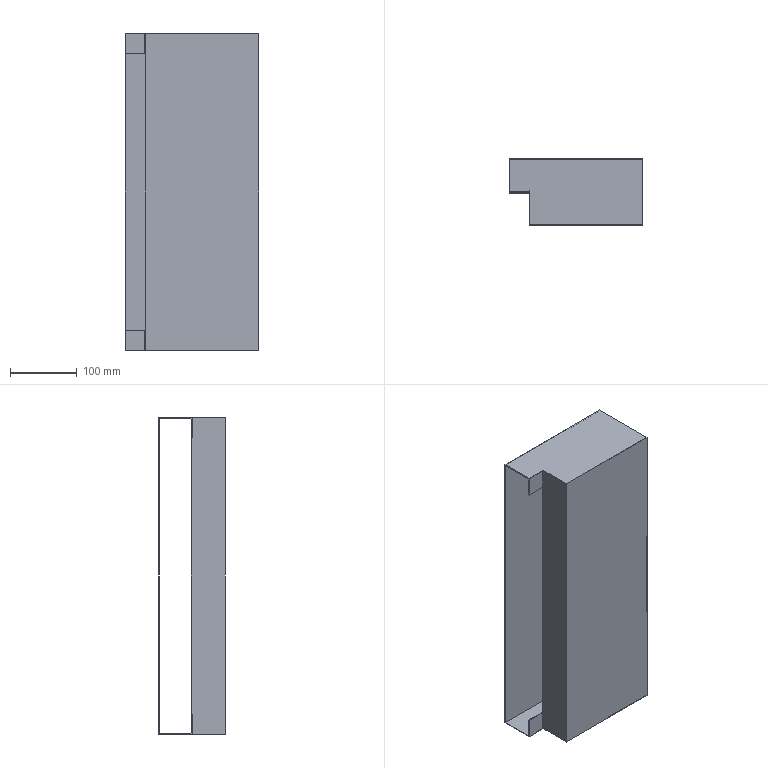Part | SolidWorks | features BaseBody 1 | 1 solid | 23 faces | box 200 x 100 x 472.4 mm | volume 283368 mm3 | plane 23
STEP:
#1=CARTESIAN_POINT('',(-200.,48.8,-236.2));
#2=VERTEX_POINT('',#1);
#3=CARTESIAN_POINT('',(-171.,48.8,-236.2));
#4=VERTEX_POINT('',#3);
#5=CARTESIAN_POINT('',(-171.,48.8,-236.2));
#6=DIRECTION('',(1.,0.,0.));
#7=VECTOR('',#6,1000.);
#8=LINE('',#5,#7);
#9=EDGE_CURVE('',#2,#4,#8,.T.);
#10=ORIENTED_EDGE('',*,*,#9,.T.);
#11=CARTESIAN_POINT('',(-171.,48.8,-206.2));
#12=VERTEX_POINT('',#11);
#13=CARTESIAN_POINT('',(-171.,48.8,-236.2));
#14=DIRECTION('',(0.,0.,1.));
#15=VECTOR('',#14,1000.);
#16=LINE('',#13,#15);
#17=EDGE_CURVE('',#4,#12,#16,.T.);
#18=ORIENTED_EDGE('',*,*,#17,.T.);
#19=CARTESIAN_POINT('',(-200.,48.8,-206.2));
#20=VERTEX_POINT('',#19);
#21=CARTESIAN_POINT('',(-171.,48.8,-206.2));
#22=DIRECTION('',(-1.,0.,0.));
#23=VECTOR('',#22,1000.);
#24=LINE('',#21,#23);
#25=EDGE_CURVE('',#12,#20,#24,.T.);
#26=ORIENTED_EDGE('',*,*,#25,.T.);
#27=CARTESIAN_POINT('',(-200.,48.8,-236.2));
#28=DIRECTION('',(0.,0.,-1.));
#29=VECTOR('',#28,1000.);
#30=LINE('',#27,#29);
#31=EDGE_CURVE('',#20,#2,#30,.T.);
#32=ORIENTED_EDGE('',*,*,#31,.T.);
#33=EDGE_LOOP('',(#10,#18,#26,#32));
#34=FACE_OUTER_BOUND('',#33,.T.);
#35=CARTESIAN_POINT('',(0.,48.8,0.));
#36=DIRECTION('',(0.,1.,0.));
#37=DIRECTION('',(1.,0.,0.));
#38=AXIS2_PLACEMENT_3D('',#35,#36,#37);
#39=PLANE('',#38);
#40=ADVANCED_FACE('',(#34),#39,.F.);
#41=CARTESIAN_POINT('',(-171.,50.,-206.2));
#42=VERTEX_POINT('',#41);
#43=CARTESIAN_POINT('',(-200.,50.,-206.2));
#44=VERTEX_POINT('',#43);
#45=CARTESIAN_POINT('',(-171.,50.,-206.2));
#46=DIRECTION('',(-1.,0.,0.));
#47=VECTOR('',#46,1000.);
#48=LINE('',#45,#47);
#49=EDGE_CURVE('',#42,#44,#48,.T.);
#50=ORIENTED_EDGE('',*,*,#49,.T.);
#51=CARTESIAN_POINT('',(-200.,48.8,-206.2));
#52=DIRECTION('',(0.,1.,0.));
#53=VECTOR('',#52,1000.);
#54=LINE('',#51,#53);
#55=EDGE_CURVE('',#20,#44,#54,.T.);
#56=ORIENTED_EDGE('',*,*,#55,.F.);
#57=ORIENTED_EDGE('',*,*,#25,.F.);
#58=CARTESIAN_POINT('',(-171.,48.8,-206.2));
#59=DIRECTION('',(0.,1.,0.));
#60=VECTOR('',#59,1000.);
#61=LINE('',#58,#60);
#62=EDGE_CURVE('',#12,#42,#61,.T.);
#63=ORIENTED_EDGE('',*,*,#62,.T.);
#64=EDGE_LOOP('',(#50,#56,#57,#63));
#65=FACE_OUTER_BOUND('',#64,.T.);
#66=CARTESIAN_POINT('',(-171.,48.8,-206.2));
#67=DIRECTION('',(0.,0.,-1.));
#68=DIRECTION('',(0.,-1.,0.));
#69=AXIS2_PLACEMENT_3D('',#66,#67,#68);
#70=PLANE('',#69);
#71=ADVANCED_FACE('',(#65),#70,.F.);
#72=CARTESIAN_POINT('',(-171.,50.,-236.2));
#73=VERTEX_POINT('',#72);
#74=CARTESIAN_POINT('',(-171.,50.,-235.));
#75=VERTEX_POINT('',#74);
#76=CARTESIAN_POINT('',(-171.,50.,-236.2));
#77=DIRECTION('',(0.,0.,1.));
#78=VECTOR('',#77,1000.);
#79=LINE('',#76,#78);
#80=EDGE_CURVE('',#73,#75,#79,.T.);
#81=ORIENTED_EDGE('',*,*,#80,.T.);
#82=CARTESIAN_POINT('',(-171.,50.,-236.2));
#83=DIRECTION('',(0.,0.,1.));
#84=VECTOR('',#83,1000.);
#85=LINE('',#82,#84);
#86=EDGE_CURVE('',#75,#42,#85,.T.);
#87=ORIENTED_EDGE('',*,*,#86,.T.);
#88=ORIENTED_EDGE('',*,*,#62,.F.);
#89=ORIENTED_EDGE('',*,*,#17,.F.);
#90=CARTESIAN_POINT('',(-171.,48.8,-236.2));
#91=DIRECTION('',(0.,1.,0.));
#92=VECTOR('',#91,1000.);
#93=LINE('',#90,#92);
#94=EDGE_CURVE('',#4,#73,#93,.T.);
#95=ORIENTED_EDGE('',*,*,#94,.T.);
#96=EDGE_LOOP('',(#81,#87,#88,#89,#95));
#97=FACE_OUTER_BOUND('',#96,.T.);
#98=CARTESIAN_POINT('',(-171.,48.8,-236.2));
#99=DIRECTION('',(-1.,0.,0.));
#100=DIRECTION('',(0.,1.,0.));
#101=AXIS2_PLACEMENT_3D('',#98,#99,#100);
#102=PLANE('',#101);
#103=ADVANCED_FACE('',(#97),#102,.F.);
#104=CARTESIAN_POINT('',(-200.,50.,-235.));
#105=VERTEX_POINT('',#104);
#106=CARTESIAN_POINT('',(-200.,50.,-235.));
#107=DIRECTION('',(1.,0.,0.));
#108=VECTOR('',#107,1000.);
#109=LINE('',#106,#108);
#110=EDGE_CURVE('',#105,#75,#109,.T.);
#111=ORIENTED_EDGE('',*,*,#110,.F.);
#112=CARTESIAN_POINT('',(-200.,50.,-236.2));
#113=DIRECTION('',(0.,0.,-1.));
#114=VECTOR('',#113,1000.);
#115=LINE('',#112,#114);
#116=EDGE_CURVE('',#44,#105,#115,.T.);
#117=ORIENTED_EDGE('',*,*,#116,.F.);
#118=ORIENTED_EDGE('',*,*,#49,.F.);
#119=ORIENTED_EDGE('',*,*,#86,.F.);
#120=EDGE_LOOP('',(#111,#117,#118,#119));
#121=FACE_OUTER_BOUND('',#120,.T.);
#122=CARTESIAN_POINT('',(0.,50.,0.));
#123=DIRECTION('',(0.,1.,0.));
#124=DIRECTION('',(1.,0.,0.));
#125=AXIS2_PLACEMENT_3D('',#122,#123,#124);
#126=PLANE('',#125);
#127=ADVANCED_FACE('',(#121),#126,.T.);
#128=CARTESIAN_POINT('',(-200.,50.,235.));
#129=VERTEX_POINT('',#128);
#130=CARTESIAN_POINT('',(-200.,50.,206.2));
#131=VERTEX_POINT('',#130);
#132=CARTESIAN_POINT('',(-200.,50.,236.2));
#133=DIRECTION('',(0.,0.,-1.));
#134=VECTOR('',#133,1000.);
#135=LINE('',#132,#134);
#136=EDGE_CURVE('',#129,#131,#135,.T.);
#137=ORIENTED_EDGE('',*,*,#136,.F.);
#138=CARTESIAN_POINT('',(-171.,50.,235.));
#139=VERTEX_POINT('',#138);
#140=CARTESIAN_POINT('',(-200.,50.,235.));
#141=DIRECTION('',(-1.,0.,0.));
#142=VECTOR('',#141,1000.);
#143=LINE('',#140,#142);
#144=EDGE_CURVE('',#139,#129,#143,.T.);
#145=ORIENTED_EDGE('',*,*,#144,.F.);
#146=CARTESIAN_POINT('',(-171.,50.,206.2));
#147=VERTEX_POINT('',#146);
#148=CARTESIAN_POINT('',(-171.,50.,236.2));
#149=DIRECTION('',(0.,0.,1.));
#150=VECTOR('',#149,1000.);
#151=LINE('',#148,#150);
#152=EDGE_CURVE('',#147,#139,#151,.T.);
#153=ORIENTED_EDGE('',*,*,#152,.F.);
#154=CARTESIAN_POINT('',(-171.,50.,206.2));
#155=DIRECTION('',(1.,0.,0.));
#156=VECTOR('',#155,1000.);
#157=LINE('',#154,#156);
#158=EDGE_CURVE('',#131,#147,#157,.T.);
#159=ORIENTED_EDGE('',*,*,#158,.F.);
#160=EDGE_LOOP('',(#137,#145,#153,#159));
#161=FACE_OUTER_BOUND('',#160,.T.);
#162=CARTESIAN_POINT('',(0.,50.,0.));
#163=DIRECTION('',(0.,1.,0.));
#164=DIRECTION('',(1.,0.,0.));
#165=AXIS2_PLACEMENT_3D('',#162,#163,#164);
#166=PLANE('',#165);
#167=ADVANCED_FACE('',(#161),#166,.T.);
#168=CARTESIAN_POINT('',(-171.,48.8,206.2));
#169=VERTEX_POINT('',#168);
#170=CARTESIAN_POINT('',(-171.,48.8,236.2));
#171=VERTEX_POINT('',#170);
#172=CARTESIAN_POINT('',(-171.,48.8,236.2));
#173=DIRECTION('',(0.,0.,1.));
#174=VECTOR('',#173,1000.);
#175=LINE('',#172,#174);
#176=EDGE_CURVE('',#169,#171,#175,.T.);
#177=ORIENTED_EDGE('',*,*,#176,.T.);
#178=CARTESIAN_POINT('',(-200.,48.8,236.2));
#179=VERTEX_POINT('',#178);
#180=CARTESIAN_POINT('',(-171.,48.8,236.2));
#181=DIRECTION('',(-1.,0.,0.));
#182=VECTOR('',#181,1000.);
#183=LINE('',#180,#182);
#184=EDGE_CURVE('',#171,#179,#183,.T.);
#185=ORIENTED_EDGE('',*,*,#184,.T.);
#186=CARTESIAN_POINT('',(-200.,48.8,206.2));
#187=VERTEX_POINT('',#186);
#188=CARTESIAN_POINT('',(-200.,48.8,236.2));
#189=DIRECTION('',(0.,0.,-1.));
#190=VECTOR('',#189,1000.);
#191=LINE('',#188,#190);
#192=EDGE_CURVE('',#179,#187,#191,.T.);
#193=ORIENTED_EDGE('',*,*,#192,.T.);
#194=CARTESIAN_POINT('',(-171.,48.8,206.2));
#195=DIRECTION('',(1.,0.,0.));
#196=VECTOR('',#195,1000.);
#197=LINE('',#194,#196);
#198=EDGE_CURVE('',#187,#169,#197,.T.);
#199=ORIENTED_EDGE('',*,*,#198,.T.);
#200=EDGE_LOOP('',(#177,#185,#193,#199));
#201=FACE_OUTER_BOUND('',#200,.T.);
#202=CARTESIAN_POINT('',(0.,48.8,0.));
#203=DIRECTION('',(0.,1.,0.));
#204=DIRECTION('',(1.,0.,0.));
#205=AXIS2_PLACEMENT_3D('',#202,#203,#204);
#206=PLANE('',#205);
#207=ADVANCED_FACE('',(#201),#206,.F.);
#208=ORIENTED_EDGE('',*,*,#158,.T.);
#209=CARTESIAN_POINT('',(-171.,48.8,206.2));
#210=DIRECTION('',(0.,1.,0.));
#211=VECTOR('',#210,1000.);
#212=LINE('',#209,#211);
#213=EDGE_CURVE('',#169,#147,#212,.T.);
#214=ORIENTED_EDGE('',*,*,#213,.F.);
#215=ORIENTED_EDGE('',*,*,#198,.F.);
#216=CARTESIAN_POINT('',(-200.,48.8,206.2));
#217=DIRECTION('',(0.,1.,0.));
#218=VECTOR('',#217,1000.);
#219=LINE('',#216,#218);
#220=EDGE_CURVE('',#187,#131,#219,.T.);
#221=ORIENTED_EDGE('',*,*,#220,.T.);
#222=EDGE_LOOP('',(#208,#214,#215,#221));
#223=FACE_OUTER_BOUND('',#222,.T.);
#224=CARTESIAN_POINT('',(-171.,48.8,206.2));
#225=DIRECTION('',(0.,0.,1.));
#226=DIRECTION('',(1.,0.,0.));
#227=AXIS2_PLACEMENT_3D('',#224,#225,#226);
#228=PLANE('',#227);
#229=ADVANCED_FACE('',(#223),#228,.F.);
#230=ORIENTED_EDGE('',*,*,#152,.T.);
#231=CARTESIAN_POINT('',(-171.,50.,236.2));
#232=VERTEX_POINT('',#231);
#233=CARTESIAN_POINT('',(-171.,50.,236.2));
#234=DIRECTION('',(0.,0.,1.));
#235=VECTOR('',#234,1000.);
#236=LINE('',#233,#235);
#237=EDGE_CURVE('',#139,#232,#236,.T.);
#238=ORIENTED_EDGE('',*,*,#237,.T.);
#239=CARTESIAN_POINT('',(-171.,48.8,236.2));
#240=DIRECTION('',(0.,1.,0.));
#241=VECTOR('',#240,1000.);
#242=LINE('',#239,#241);
#243=EDGE_CURVE('',#171,#232,#242,.T.);
#244=ORIENTED_EDGE('',*,*,#243,.F.);
#245=ORIENTED_EDGE('',*,*,#176,.F.);
#246=ORIENTED_EDGE('',*,*,#213,.T.);
#247=EDGE_LOOP('',(#230,#238,#244,#245,#246));
#248=FACE_OUTER_BOUND('',#247,.T.);
#249=CARTESIAN_POINT('',(-171.,48.8,236.2));
#250=DIRECTION('',(-1.,0.,0.));
#251=DIRECTION('',(0.,1.,0.));
#252=AXIS2_PLACEMENT_3D('',#249,#250,#251);
#253=PLANE('',#252);
#254=ADVANCED_FACE('',(#248),#253,.F.);
#255=CARTESIAN_POINT('',(-168.8,1.2,-235.));
#256=VERTEX_POINT('',#255);
#257=CARTESIAN_POINT('',(-168.8,1.2,235.));
#258=VERTEX_POINT('',#257);
#259=CARTESIAN_POINT('',(-168.8,1.2,-294.51));
#260=DIRECTION('',(0.,0.,1.));
#261=VECTOR('',#260,1000.);
#262=LINE('',#259,#261);
#263=EDGE_CURVE('',#256,#258,#262,.T.);
#264=ORIENTED_EDGE('',*,*,#263,.F.);
#265=CARTESIAN_POINT('',(-168.8,51.2,-235.));
#266=VERTEX_POINT('',#265);
#267=CARTESIAN_POINT('',(-168.8,0.,-235.));
#268=DIRECTION('',(0.,1.,0.));
#269=VECTOR('',#268,1000.);
#270=LINE('',#267,#269);
#271=EDGE_CURVE('',#256,#266,#270,.T.);
#272=ORIENTED_EDGE('',*,*,#271,.T.);
#273=CARTESIAN_POINT('',(-168.8,51.2,235.));
#274=VERTEX_POINT('',#273);
#275=CARTESIAN_POINT('',(-168.8,51.2,-294.51));
#276=DIRECTION('',(0.,0.,1.));
#277=VECTOR('',#276,1000.);
#278=LINE('',#275,#277);
#279=EDGE_CURVE('',#266,#274,#278,.T.);
#280=ORIENTED_EDGE('',*,*,#279,.T.);
#281=CARTESIAN_POINT('',(-168.8,0.,235.));
#282=DIRECTION('',(0.,1.,0.));
#283=VECTOR('',#282,1000.);
#284=LINE('',#281,#283);
#285=EDGE_CURVE('',#258,#274,#284,.T.);
#286=ORIENTED_EDGE('',*,*,#285,.F.);
#287=EDGE_LOOP('',(#264,#272,#280,#286));
#288=FACE_OUTER_BOUND('',#287,.T.);
#289=CARTESIAN_POINT('',(-168.8,0.,-294.51));
#290=DIRECTION('',(1.,0.,0.));
#291=DIRECTION('',(0.,1.,0.));
#292=AXIS2_PLACEMENT_3D('',#289,#290,#291);
#293=PLANE('',#292);
#294=ADVANCED_FACE('',(#288),#293,.T.);
#295=CARTESIAN_POINT('',(-170.,51.2,235.));
#296=VERTEX_POINT('',#295);
#297=CARTESIAN_POINT('',(-170.,51.2,-235.));
#298=VERTEX_POINT('',#297);
#299=CARTESIAN_POINT('',(-170.,51.2,-294.51));
#300=DIRECTION('',(0.,0.,-1.));
#301=VECTOR('',#300,1000.);
#302=LINE('',#299,#301);
#303=EDGE_CURVE('',#296,#298,#302,.T.);
#304=ORIENTED_EDGE('',*,*,#303,.F.);
#305=CARTESIAN_POINT('',(-170.,51.2,235.));
#306=DIRECTION('',(-1.,0.,0.));
#307=VECTOR('',#306,1000.);
#308=LINE('',#305,#307);
#309=EDGE_CURVE('',#274,#296,#308,.T.);
#310=ORIENTED_EDGE('',*,*,#309,.F.);
#311=ORIENTED_EDGE('',*,*,#279,.F.);
#312=CARTESIAN_POINT('',(-170.,51.2,-235.));
#313=DIRECTION('',(-1.,0.,0.));
#314=VECTOR('',#313,1000.);
#315=LINE('',#312,#314);
#316=EDGE_CURVE('',#266,#298,#315,.T.);
#317=ORIENTED_EDGE('',*,*,#316,.T.);
#318=EDGE_LOOP('',(#304,#310,#311,#317));
#319=FACE_OUTER_BOUND('',#318,.T.);
#320=CARTESIAN_POINT('',(-170.,51.2,-294.51));
#321=DIRECTION('',(0.,1.,0.));
#322=DIRECTION('',(1.,0.,0.));
#323=AXIS2_PLACEMENT_3D('',#320,#321,#322);
#324=PLANE('',#323);
#325=ADVANCED_FACE('',(#319),#324,.T.);
#326=CARTESIAN_POINT('',(0.,98.8,-235.));
#327=VERTEX_POINT('',#326);
#328=CARTESIAN_POINT('',(-200.,98.8,-235.));
#329=VERTEX_POINT('',#328);
#330=CARTESIAN_POINT('',(0.,98.8,-235.));
#331=DIRECTION('',(-1.,0.,0.));
#332=VECTOR('',#331,1000.);
#333=LINE('',#330,#332);
#334=EDGE_CURVE('',#327,#329,#333,.T.);
#335=ORIENTED_EDGE('',*,*,#334,.T.);
#336=CARTESIAN_POINT('',(-200.,569.756,-235.));
#337=DIRECTION('',(0.,-1.,0.));
#338=VECTOR('',#337,1000.);
#339=LINE('',#336,#338);
#340=EDGE_CURVE('',#329,#105,#339,.T.);
#341=ORIENTED_EDGE('',*,*,#340,.T.);
#342=ORIENTED_EDGE('',*,*,#110,.T.);
#343=CARTESIAN_POINT('',(-170.,50.,-235.));
#344=VERTEX_POINT('',#343);
#345=CARTESIAN_POINT('',(-200.,50.,-235.));
#346=DIRECTION('',(1.,0.,0.));
#347=VECTOR('',#346,1000.);
#348=LINE('',#345,#347);
#349=EDGE_CURVE('',#75,#344,#348,.T.);
#350=ORIENTED_EDGE('',*,*,#349,.T.);
#351=CARTESIAN_POINT('',(-170.,569.756,-235.));
#352=DIRECTION('',(0.,-1.,0.));
#353=VECTOR('',#352,1000.);
#354=LINE('',#351,#353);
#355=EDGE_CURVE('',#298,#344,#354,.T.);
#356=ORIENTED_EDGE('',*,*,#355,.F.);
#357=ORIENTED_EDGE('',*,*,#316,.F.);
#358=ORIENTED_EDGE('',*,*,#271,.F.);
#359=CARTESIAN_POINT('',(0.,1.2,-235.));
#360=VERTEX_POINT('',#359);
#361=CARTESIAN_POINT('',(0.,1.2,-235.));
#362=DIRECTION('',(1.,0.,0.));
#363=VECTOR('',#362,1000.);
#364=LINE('',#361,#363);
#365=EDGE_CURVE('',#256,#360,#364,.T.);
#366=ORIENTED_EDGE('',*,*,#365,.T.);
#367=CARTESIAN_POINT('',(0.,0.,-235.));
#368=DIRECTION('',(0.,1.,0.));
#369=VECTOR('',#368,1000.);
#370=LINE('',#367,#369);
#371=EDGE_CURVE('',#360,#327,#370,.T.);
#372=ORIENTED_EDGE('',*,*,#371,.T.);
#373=EDGE_LOOP('',(#335,#341,#342,#350,#356,#357,#358,#366,#372));
#374=FACE_OUTER_BOUND('',#373,.T.);
#375=CARTESIAN_POINT('',(0.,0.,-235.));
#376=DIRECTION('',(0.,0.,-1.));
#377=DIRECTION('',(0.,-1.,0.));
#378=AXIS2_PLACEMENT_3D('',#375,#376,#377);
#379=PLANE('',#378);
#380=ADVANCED_FACE('',(#374),#379,.F.);
#381=ORIENTED_EDGE('',*,*,#309,.T.);
#382=CARTESIAN_POINT('',(-170.,50.,235.));
#383=VERTEX_POINT('',#382);
#384=CARTESIAN_POINT('',(-170.,569.756,235.));
#385=DIRECTION('',(0.,-1.,0.));
#386=VECTOR('',#385,1000.);
#387=LINE('',#384,#386);
#388=EDGE_CURVE('',#296,#383,#387,.T.);
#389=ORIENTED_EDGE('',*,*,#388,.T.);
#390=CARTESIAN_POINT('',(-200.,50.,235.));
#391=DIRECTION('',(-1.,0.,0.));
#392=VECTOR('',#391,1000.);
#393=LINE('',#390,#392);
#394=EDGE_CURVE('',#383,#139,#393,.T.);
#395=ORIENTED_EDGE('',*,*,#394,.T.);
#396=ORIENTED_EDGE('',*,*,#144,.T.);
#397=CARTESIAN_POINT('',(-200.,98.8,235.));
#398=VERTEX_POINT('',#397);
#399=CARTESIAN_POINT('',(-200.,569.756,235.));
#400=DIRECTION('',(0.,-1.,0.));
#401=VECTOR('',#400,1000.);
#402=LINE('',#399,#401);
#403=EDGE_CURVE('',#398,#129,#402,.T.);
#404=ORIENTED_EDGE('',*,*,#403,.F.);
#405=CARTESIAN_POINT('',(0.,98.8,235.));
#406=VERTEX_POINT('',#405);
#407=CARTESIAN_POINT('',(0.,98.8,235.));
#408=DIRECTION('',(-1.,0.,0.));
#409=VECTOR('',#408,1000.);
#410=LINE('',#407,#409);
#411=EDGE_CURVE('',#406,#398,#410,.T.);
#412=ORIENTED_EDGE('',*,*,#411,.F.);
#413=CARTESIAN_POINT('',(0.,1.2,235.));
#414=VERTEX_POINT('',#413);
#415=CARTESIAN_POINT('',(0.,0.,235.));
#416=DIRECTION('',(0.,1.,0.));
#417=VECTOR('',#416,1000.);
#418=LINE('',#415,#417);
#419=EDGE_CURVE('',#414,#406,#418,.T.);
#420=ORIENTED_EDGE('',*,*,#419,.F.);
#421=CARTESIAN_POINT('',(0.,1.2,235.));
#422=DIRECTION('',(1.,0.,0.));
#423=VECTOR('',#422,1000.);
#424=LINE('',#421,#423);
#425=EDGE_CURVE('',#258,#414,#424,.T.);
#426=ORIENTED_EDGE('',*,*,#425,.F.);
#427=ORIENTED_EDGE('',*,*,#285,.T.);
#428=EDGE_LOOP('',(#381,#389,#395,#396,#404,#412,#420,#426,#427));
#429=FACE_OUTER_BOUND('',#428,.T.);
#430=CARTESIAN_POINT('',(0.,0.,235.));
#431=DIRECTION('',(0.,0.,-1.));
#432=DIRECTION('',(0.,-1.,0.));
#433=AXIS2_PLACEMENT_3D('',#430,#431,#432);
#434=PLANE('',#433);
#435=ADVANCED_FACE('',(#429),#434,.T.);
#436=ORIENTED_EDGE('',*,*,#425,.T.);
#437=CARTESIAN_POINT('',(0.,1.2,236.2));
#438=DIRECTION('',(0.,0.,-1.));
#439=VECTOR('',#438,1000.);
#440=LINE('',#437,#439);
#441=EDGE_CURVE('',#414,#360,#440,.T.);
#442=ORIENTED_EDGE('',*,*,#441,.T.);
#443=ORIENTED_EDGE('',*,*,#365,.F.);
#444=ORIENTED_EDGE('',*,*,#263,.T.);
#445=EDGE_LOOP('',(#436,#442,#443,#444));
#446=FACE_OUTER_BOUND('',#445,.T.);
#447=CARTESIAN_POINT('',(0.,1.2,236.2));
#448=DIRECTION('',(0.,1.,0.));
#449=DIRECTION('',(1.,0.,0.));
#450=AXIS2_PLACEMENT_3D('',#447,#448,#449);
#451=PLANE('',#450);
#452=ADVANCED_FACE('',(#446),#451,.T.);
#453=ORIENTED_EDGE('',*,*,#411,.T.);
#454=CARTESIAN_POINT('',(-200.,98.8,235.));
#455=DIRECTION('',(0.,0.,1.));
#456=VECTOR('',#455,1000.);
#457=LINE('',#454,#456);
#458=EDGE_CURVE('',#329,#398,#457,.T.);
#459=ORIENTED_EDGE('',*,*,#458,.F.);
#460=ORIENTED_EDGE('',*,*,#334,.F.);
#461=CARTESIAN_POINT('',(0.,98.8,236.2));
#462=DIRECTION('',(0.,0.,-1.));
#463=VECTOR('',#462,1000.);
#464=LINE('',#461,#463);
#465=EDGE_CURVE('',#406,#327,#464,.T.);
#466=ORIENTED_EDGE('',*,*,#465,.F.);
#467=EDGE_LOOP('',(#453,#459,#460,#466));
#468=FACE_OUTER_BOUND('',#467,.T.);
#469=CARTESIAN_POINT('',(-200.,98.8,236.2));
#470=DIRECTION('',(0.,-1.,0.));
#471=DIRECTION('',(0.,0.,-1.));
#472=AXIS2_PLACEMENT_3D('',#469,#470,#471);
#473=PLANE('',#472);
#474=ADVANCED_FACE('',(#468),#473,.T.);
#475=CARTESIAN_POINT('',(-170.,0.,-236.2));
#476=VERTEX_POINT('',#475);
#477=CARTESIAN_POINT('',(-170.,0.,236.2));
#478=VERTEX_POINT('',#477);
#479=CARTESIAN_POINT('',(-170.,0.,-294.51));
#480=DIRECTION('',(0.,0.,1.));
#481=VECTOR('',#480,1000.);
#482=LINE('',#479,#481);
#483=EDGE_CURVE('',#476,#478,#482,.T.);
#484=ORIENTED_EDGE('',*,*,#483,.T.);
#485=CARTESIAN_POINT('',(-170.,50.,236.2));
#486=VERTEX_POINT('',#485);
#487=CARTESIAN_POINT('',(-170.,0.,236.2));
#488=DIRECTION('',(0.,1.,0.));
#489=VECTOR('',#488,1000.);
#490=LINE('',#487,#489);
#491=EDGE_CURVE('',#478,#486,#490,.T.);
#492=ORIENTED_EDGE('',*,*,#491,.T.);
#493=CARTESIAN_POINT('',(-170.,50.,-294.51));
#494=DIRECTION('',(0.,0.,1.));
#495=VECTOR('',#494,1000.);
#496=LINE('',#493,#495);
#497=EDGE_CURVE('',#383,#486,#496,.T.);
#498=ORIENTED_EDGE('',*,*,#497,.F.);
#499=ORIENTED_EDGE('',*,*,#388,.F.);
#500=ORIENTED_EDGE('',*,*,#303,.T.);
#501=ORIENTED_EDGE('',*,*,#355,.T.);
#502=CARTESIAN_POINT('',(-170.,50.,-236.2));
#503=VERTEX_POINT('',#502);
#504=CARTESIAN_POINT('',(-170.,50.,-294.51));
#505=DIRECTION('',(0.,0.,1.));
#506=VECTOR('',#505,1000.);
#507=LINE('',#504,#506);
#508=EDGE_CURVE('',#503,#344,#507,.T.);
#509=ORIENTED_EDGE('',*,*,#508,.F.);
#510=CARTESIAN_POINT('',(-170.,0.,-236.2));
#511=DIRECTION('',(0.,1.,0.));
#512=VECTOR('',#511,1000.);
#513=LINE('',#510,#512);
#514=EDGE_CURVE('',#476,#503,#513,.T.);
#515=ORIENTED_EDGE('',*,*,#514,.F.);
#516=EDGE_LOOP('',(#484,#492,#498,#499,#500,#501,#509,#515));
#517=FACE_OUTER_BOUND('',#516,.T.);
#518=CARTESIAN_POINT('',(-170.,0.,-294.51));
#519=DIRECTION('',(1.,0.,0.));
#520=DIRECTION('',(0.,1.,0.));
#521=AXIS2_PLACEMENT_3D('',#518,#519,#520);
#522=PLANE('',#521);
#523=ADVANCED_FACE('',(#517),#522,.F.);
#524=CARTESIAN_POINT('',(-170.,50.,-236.2));
#525=DIRECTION('',(-1.,0.,0.));
#526=VECTOR('',#525,1000.);
#527=LINE('',#524,#526);
#528=EDGE_CURVE('',#503,#73,#527,.T.);
#529=ORIENTED_EDGE('',*,*,#528,.T.);
#530=ORIENTED_EDGE('',*,*,#94,.F.);
#531=ORIENTED_EDGE('',*,*,#9,.F.);
#532=CARTESIAN_POINT('',(-200.,100.,-236.2));
#533=VERTEX_POINT('',#532);
#534=CARTESIAN_POINT('',(-200.,0.,-236.2));
#535=DIRECTION('',(0.,-1.,0.));
#536=VECTOR('',#535,1000.);
#537=LINE('',#534,#536);
#538=EDGE_CURVE('',#533,#2,#537,.T.);
#539=ORIENTED_EDGE('',*,*,#538,.F.);
#540=CARTESIAN_POINT('',(0.,100.,-236.2));
#541=VERTEX_POINT('',#540);
#542=CARTESIAN_POINT('',(-200.,100.,-236.2));
#543=DIRECTION('',(-1.,0.,0.));
#544=VECTOR('',#543,1000.);
#545=LINE('',#542,#544);
#546=EDGE_CURVE('',#541,#533,#545,.T.);
#547=ORIENTED_EDGE('',*,*,#546,.F.);
#548=CARTESIAN_POINT('',(0.,0.,-236.2));
#549=VERTEX_POINT('',#548);
#550=CARTESIAN_POINT('',(0.,100.,-236.2));
#551=DIRECTION('',(0.,1.,0.));
#552=VECTOR('',#551,1000.);
#553=LINE('',#550,#552);
#554=EDGE_CURVE('',#549,#541,#553,.T.);
#555=ORIENTED_EDGE('',*,*,#554,.F.);
#556=CARTESIAN_POINT('',(0.,0.,-236.2));
#557=DIRECTION('',(1.,0.,0.));
#558=VECTOR('',#557,1000.);
#559=LINE('',#556,#558);
#560=EDGE_CURVE('',#476,#549,#559,.T.);
#561=ORIENTED_EDGE('',*,*,#560,.F.);
#562=ORIENTED_EDGE('',*,*,#514,.T.);
#563=EDGE_LOOP('',(#529,#530,#531,#539,#547,#555,#561,#562));
#564=FACE_OUTER_BOUND('',#563,.T.);
#565=CARTESIAN_POINT('',(0.,0.,-236.2));
#566=DIRECTION('',(0.,0.,-1.));
#567=DIRECTION('',(0.,-1.,0.));
#568=AXIS2_PLACEMENT_3D('',#565,#566,#567);
#569=PLANE('',#568);
#570=ADVANCED_FACE('',(#564),#569,.T.);
#571=CARTESIAN_POINT('',(-200.,100.,236.2));
#572=VERTEX_POINT('',#571);
#573=CARTESIAN_POINT('',(-200.,0.,236.2));
#574=DIRECTION('',(0.,-1.,0.));
#575=VECTOR('',#574,1000.);
#576=LINE('',#573,#575);
#577=EDGE_CURVE('',#572,#179,#576,.T.);
#578=ORIENTED_EDGE('',*,*,#577,.T.);
#579=ORIENTED_EDGE('',*,*,#184,.F.);
#580=ORIENTED_EDGE('',*,*,#243,.T.);
#581=CARTESIAN_POINT('',(-170.,50.,236.2));
#582=DIRECTION('',(-1.,0.,0.));
#583=VECTOR('',#582,1000.);
#584=LINE('',#581,#583);
#585=EDGE_CURVE('',#486,#232,#584,.T.);
#586=ORIENTED_EDGE('',*,*,#585,.F.);
#587=ORIENTED_EDGE('',*,*,#491,.F.);
#588=CARTESIAN_POINT('',(0.,0.,236.2));
#589=VERTEX_POINT('',#588);
#590=CARTESIAN_POINT('',(0.,0.,236.2));
#591=DIRECTION('',(1.,0.,0.));
#592=VECTOR('',#591,1000.);
#593=LINE('',#590,#592);
#594=EDGE_CURVE('',#478,#589,#593,.T.);
#595=ORIENTED_EDGE('',*,*,#594,.T.);
#596=CARTESIAN_POINT('',(0.,100.,236.2));
#597=VERTEX_POINT('',#596);
#598=CARTESIAN_POINT('',(0.,100.,236.2));
#599=DIRECTION('',(0.,1.,0.));
#600=VECTOR('',#599,1000.);
#601=LINE('',#598,#600);
#602=EDGE_CURVE('',#589,#597,#601,.T.);
#603=ORIENTED_EDGE('',*,*,#602,.T.);
#604=CARTESIAN_POINT('',(-200.,100.,236.2));
#605=DIRECTION('',(-1.,0.,0.));
#606=VECTOR('',#605,1000.);
#607=LINE('',#604,#606);
#608=EDGE_CURVE('',#597,#572,#607,.T.);
#609=ORIENTED_EDGE('',*,*,#608,.T.);
#610=EDGE_LOOP('',(#578,#579,#580,#586,#587,#595,#603,#609));
#611=FACE_OUTER_BOUND('',#610,.T.);
#612=CARTESIAN_POINT('',(0.,0.,236.2));
#613=DIRECTION('',(0.,0.,-1.));
#614=DIRECTION('',(0.,-1.,0.));
#615=AXIS2_PLACEMENT_3D('',#612,#613,#614);
#616=PLANE('',#615);
#617=ADVANCED_FACE('',(#611),#616,.F.);
#618=ORIENTED_EDGE('',*,*,#594,.F.);
#619=ORIENTED_EDGE('',*,*,#483,.F.);
#620=ORIENTED_EDGE('',*,*,#560,.T.);
#621=CARTESIAN_POINT('',(0.,0.,236.2));
#622=DIRECTION('',(0.,0.,-1.));
#623=VECTOR('',#622,1000.);
#624=LINE('',#621,#623);
#625=EDGE_CURVE('',#589,#549,#624,.T.);
#626=ORIENTED_EDGE('',*,*,#625,.F.);
#627=EDGE_LOOP('',(#618,#619,#620,#626));
#628=FACE_OUTER_BOUND('',#627,.T.);
#629=CARTESIAN_POINT('',(0.,0.,236.2));
#630=DIRECTION('',(0.,1.,0.));
#631=DIRECTION('',(1.,0.,0.));
#632=AXIS2_PLACEMENT_3D('',#629,#630,#631);
#633=PLANE('',#632);
#634=ADVANCED_FACE('',(#628),#633,.F.);
#635=ORIENTED_EDGE('',*,*,#458,.T.);
#636=ORIENTED_EDGE('',*,*,#403,.T.);
#637=ORIENTED_EDGE('',*,*,#136,.T.);
#638=ORIENTED_EDGE('',*,*,#220,.F.);
#639=ORIENTED_EDGE('',*,*,#192,.F.);
#640=ORIENTED_EDGE('',*,*,#577,.F.);
#641=CARTESIAN_POINT('',(-200.,100.,236.2));
#642=DIRECTION('',(0.,0.,-1.));
#643=VECTOR('',#642,1000.);
#644=LINE('',#641,#643);
#645=EDGE_CURVE('',#572,#533,#644,.T.);
#646=ORIENTED_EDGE('',*,*,#645,.T.);
#647=ORIENTED_EDGE('',*,*,#538,.T.);
#648=ORIENTED_EDGE('',*,*,#31,.F.);
#649=ORIENTED_EDGE('',*,*,#55,.T.);
#650=ORIENTED_EDGE('',*,*,#116,.T.);
#651=ORIENTED_EDGE('',*,*,#340,.F.);
#652=EDGE_LOOP('',(#635,#636,#637,#638,#639,#640,#646,#647,#648,#649,#650,#651));
#653=FACE_OUTER_BOUND('',#652,.T.);
#654=CARTESIAN_POINT('',(-200.,0.,236.2));
#655=DIRECTION('',(1.,0.,0.));
#656=DIRECTION('',(0.,1.,0.));
#657=AXIS2_PLACEMENT_3D('',#654,#655,#656);
#658=PLANE('',#657);
#659=ADVANCED_FACE('',(#653),#658,.F.);
#660=ORIENTED_EDGE('',*,*,#546,.T.);
#661=ORIENTED_EDGE('',*,*,#645,.F.);
#662=ORIENTED_EDGE('',*,*,#608,.F.);
#663=CARTESIAN_POINT('',(0.,100.,236.2));
#664=DIRECTION('',(0.,0.,-1.));
#665=VECTOR('',#664,1000.);
#666=LINE('',#663,#665);
#667=EDGE_CURVE('',#597,#541,#666,.T.);
#668=ORIENTED_EDGE('',*,*,#667,.T.);
#669=EDGE_LOOP('',(#660,#661,#662,#668));
#670=FACE_OUTER_BOUND('',#669,.T.);
#671=CARTESIAN_POINT('',(-200.,100.,236.2));
#672=DIRECTION('',(0.,-1.,0.));
#673=DIRECTION('',(0.,0.,-1.));
#674=AXIS2_PLACEMENT_3D('',#671,#672,#673);
#675=PLANE('',#674);
#676=ADVANCED_FACE('',(#670),#675,.F.);
#677=ORIENTED_EDGE('',*,*,#371,.F.);
#678=ORIENTED_EDGE('',*,*,#441,.F.);
#679=ORIENTED_EDGE('',*,*,#419,.T.);
#680=ORIENTED_EDGE('',*,*,#465,.T.);
#681=EDGE_LOOP('',(#677,#678,#679,#680));
#682=FACE_BOUND('',#681,.T.);
#683=ORIENTED_EDGE('',*,*,#554,.T.);
#684=ORIENTED_EDGE('',*,*,#667,.F.);
#685=ORIENTED_EDGE('',*,*,#602,.F.);
#686=ORIENTED_EDGE('',*,*,#625,.T.);
#687=EDGE_LOOP('',(#683,#684,#685,#686));
#688=FACE_OUTER_BOUND('',#687,.T.);
#689=CARTESIAN_POINT('',(0.,100.,236.2));
#690=DIRECTION('',(-1.,0.,0.));
#691=DIRECTION('',(0.,1.,0.));
#692=AXIS2_PLACEMENT_3D('',#689,#690,#691);
#693=PLANE('',#692);
#694=ADVANCED_FACE('',(#682,#688),#693,.F.);
#695=ORIENTED_EDGE('',*,*,#237,.F.);
#696=ORIENTED_EDGE('',*,*,#394,.F.);
#697=ORIENTED_EDGE('',*,*,#497,.T.);
#698=ORIENTED_EDGE('',*,*,#585,.T.);
#699=EDGE_LOOP('',(#695,#696,#697,#698));
#700=FACE_OUTER_BOUND('',#699,.T.);
#701=CARTESIAN_POINT('',(-170.,50.,-294.51));
#702=DIRECTION('',(0.,1.,0.));
#703=DIRECTION('',(1.,0.,0.));
#704=AXIS2_PLACEMENT_3D('',#701,#702,#703);
#705=PLANE('',#704);
#706=ADVANCED_FACE('',(#700),#705,.F.);
#707=ORIENTED_EDGE('',*,*,#80,.F.);
#708=ORIENTED_EDGE('',*,*,#528,.F.);
#709=ORIENTED_EDGE('',*,*,#508,.T.);
#710=ORIENTED_EDGE('',*,*,#349,.F.);
#711=EDGE_LOOP('',(#707,#708,#709,#710));
#712=FACE_OUTER_BOUND('',#711,.T.);
#713=CARTESIAN_POINT('',(-170.,50.,-294.51));
#714=DIRECTION('',(0.,1.,0.));
#715=DIRECTION('',(1.,0.,0.));
#716=AXIS2_PLACEMENT_3D('',#713,#714,#715);
#717=PLANE('',#716);
#718=ADVANCED_FACE('',(#712),#717,.F.);
#719=CLOSED_SHELL('',(#40,#71,#103,#127,#167,#207,#229,#254,#294,#325,#380,#435,#452,#474,#523,#570,#617,#634,#659,#676,#694,#706,#718));
#720=MANIFOLD_SOLID_BREP('',#719);
#721=CARTESIAN_POINT('',(0.,0.,0.));
#722=DIRECTION('',(0.,0.,1.));
#723=DIRECTION('',(1.,0.,0.));
#724=AXIS2_PLACEMENT_3D('',#721,#722,#723);
#725=(LENGTH_UNIT()NAMED_UNIT(*)SI_UNIT(.MILLI.,.METRE.));
#726=UNCERTAINTY_MEASURE_WITH_UNIT(LENGTH_MEASURE(0.00001),#725,'','');
#727=(NAMED_UNIT(*)PLANE_ANGLE_UNIT()SI_UNIT($,.RADIAN.));
#728=(NAMED_UNIT(*)SI_UNIT($,.STERADIAN.)SOLID_ANGLE_UNIT());
#729=(GEOMETRIC_REPRESENTATION_CONTEXT(3)GLOBAL_UNCERTAINTY_ASSIGNED_CONTEXT((#726))GLOBAL_UNIT_ASSIGNED_CONTEXT((#725,#727,#728))REPRESENTATION_CONTEXT('',''));
#730=ADVANCED_BREP_SHAPE_REPRESENTATION('',(#720,#724),#729);